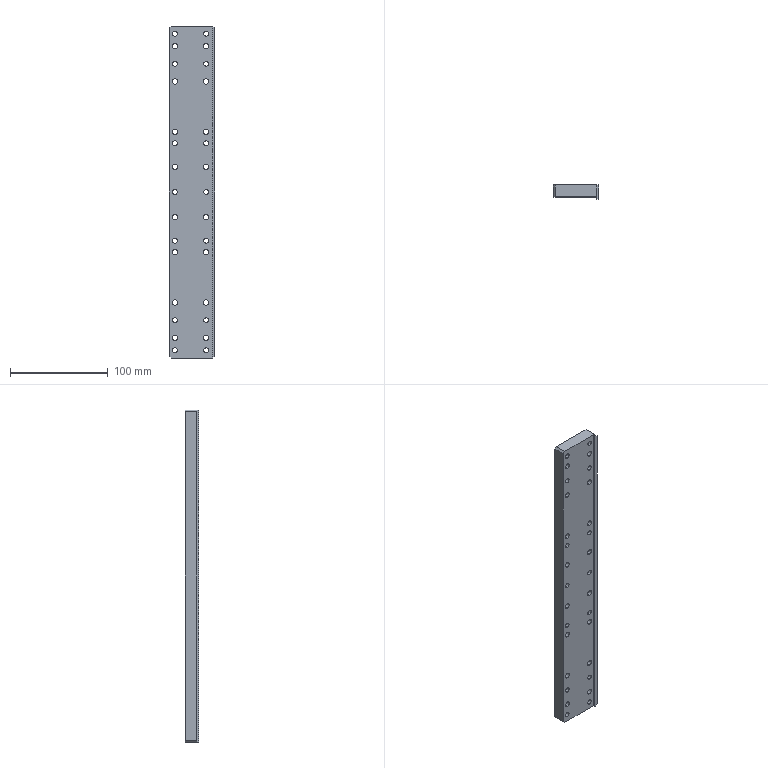Part | SolidWorks | features HoleWzd 2, Chamfer 1, Extrusion 1, MoveFace 1 | 1 solid | 120 faces | box 47 x 14 x 340 mm | volume 181103 mm3 | cylinder 92 | plane 28 | commonest cylinder face diameters 5.5 x32 10 x32 5 x28